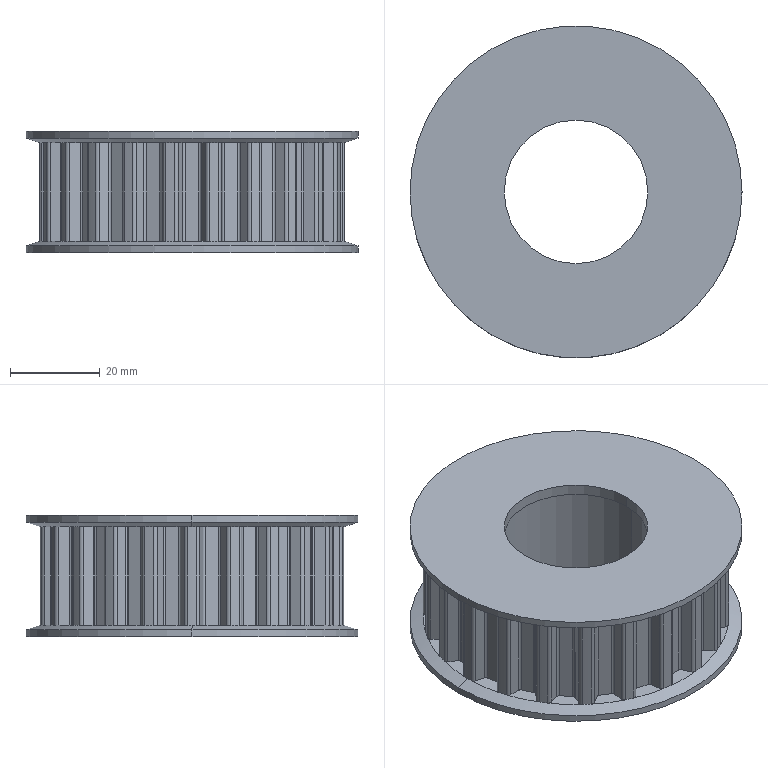Part | STEP file | Timing pulley 22-T10-φ35-27 | 1 solid | 254 faces | box 74 x 74 x 27 mm | volume 67542 mm3 | cylinder 135 | plane 113 | cone 6 | commonest cylinder face diameters 1.2 x52 1.6 x52 68.15 x23 74 x4 32 x2 35 x2